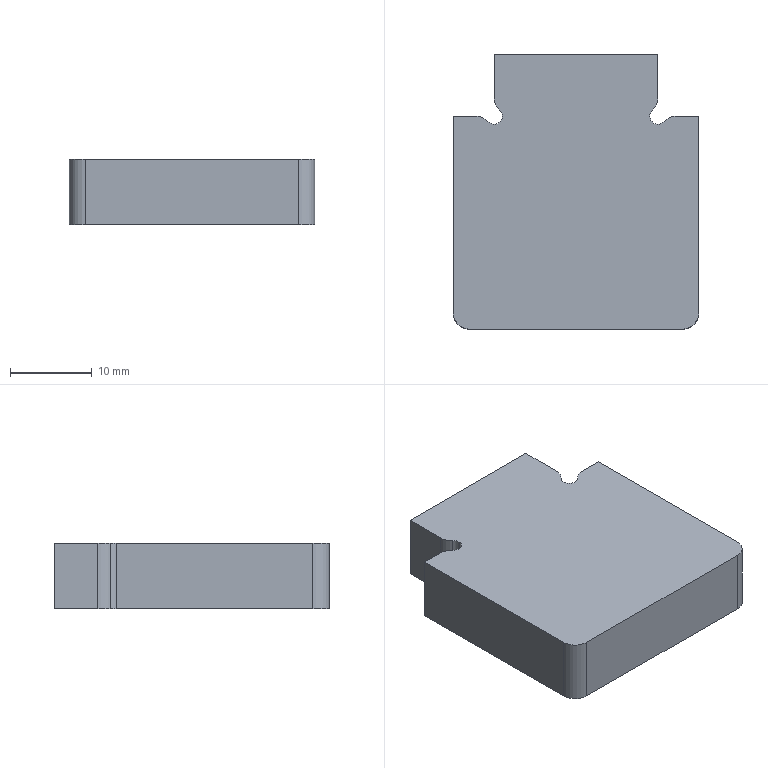Part | SolidWorks | features FlatPattern 1, SMBaseFlange 1, SheetMetal 1 | 1 solid | 19 faces | box 30 x 33.5 x 8 mm | volume 7383 mm3 | plane 10 | cylinder 9 | commonest cylinder face diameters 4 x6 2 x3
STEP:
#1=CARTESIAN_POINT('',(106.89,-100.055,-8.));
#2=VERTEX_POINT('',#1);
#3=CARTESIAN_POINT('',(107.224,-100.8,-8.));
#4=VERTEX_POINT('',#3);
#5=CARTESIAN_POINT('',(106.224,-100.8,-8.));
#6=DIRECTION('',(0.,0.,-1.));
#7=DIRECTION('',(1.,0.,0.));
#8=AXIS2_PLACEMENT_3D('',#5,#6,#7);
#9=CIRCLE('',#8,1.);
#10=EDGE_CURVE('',#2,#4,#9,.T.);
#11=ORIENTED_EDGE('',*,*,#10,.T.);
#12=CARTESIAN_POINT('',(107.224,-100.8,0.));
#13=VERTEX_POINT('',#12);
#14=CARTESIAN_POINT('',(107.224,-100.8,-8.));
#15=DIRECTION('',(0.,0.,1.));
#16=VECTOR('',#15,1000.);
#17=LINE('',#14,#16);
#18=EDGE_CURVE('',#4,#13,#17,.T.);
#19=ORIENTED_EDGE('',*,*,#18,.T.);
#20=CARTESIAN_POINT('',(106.89,-100.055,0.));
#21=VERTEX_POINT('',#20);
#22=CARTESIAN_POINT('',(106.224,-100.8,0.));
#23=DIRECTION('',(0.,0.,-1.));
#24=DIRECTION('',(1.,0.,0.));
#25=AXIS2_PLACEMENT_3D('',#22,#23,#24);
#26=CIRCLE('',#25,1.);
#27=EDGE_CURVE('',#21,#13,#26,.T.);
#28=ORIENTED_EDGE('',*,*,#27,.F.);
#29=CARTESIAN_POINT('',(106.89,-100.055,-8.));
#30=DIRECTION('',(0.,0.,1.));
#31=VECTOR('',#30,1000.);
#32=LINE('',#29,#31);
#33=EDGE_CURVE('',#2,#21,#32,.T.);
#34=ORIENTED_EDGE('',*,*,#33,.F.);
#35=EDGE_LOOP('',(#11,#19,#28,#34));
#36=FACE_OUTER_BOUND('',#35,.T.);
#37=CARTESIAN_POINT('',(106.224,-100.8,-8.));
#38=DIRECTION('',(0.,0.,1.));
#39=DIRECTION('',(1.,0.,0.));
#40=AXIS2_PLACEMENT_3D('',#37,#38,#39);
#41=CYLINDRICAL_SURFACE('',#40,1.);
#42=ADVANCED_FACE('',(#36),#41,.F.);
#43=CARTESIAN_POINT('',(103.988,-100.8,0.));
#44=VERTEX_POINT('',#43);
#45=CARTESIAN_POINT('',(101.224,-100.8,0.));
#46=VERTEX_POINT('',#45);
#47=CARTESIAN_POINT('',(103.988,-100.8,0.));
#48=DIRECTION('',(-1.,0.,0.));
#49=VECTOR('',#48,1000.);
#50=LINE('',#47,#49);
#51=EDGE_CURVE('',#44,#46,#50,.T.);
#52=ORIENTED_EDGE('',*,*,#51,.F.);
#53=CARTESIAN_POINT('',(103.988,-100.8,-8.));
#54=VERTEX_POINT('',#53);
#55=CARTESIAN_POINT('',(103.988,-100.8,-8.));
#56=DIRECTION('',(0.,0.,1.));
#57=VECTOR('',#56,1000.);
#58=LINE('',#55,#57);
#59=EDGE_CURVE('',#54,#44,#58,.T.);
#60=ORIENTED_EDGE('',*,*,#59,.F.);
#61=CARTESIAN_POINT('',(101.224,-100.8,-8.));
#62=VERTEX_POINT('',#61);
#63=CARTESIAN_POINT('',(103.988,-100.8,-8.));
#64=DIRECTION('',(-1.,0.,0.));
#65=VECTOR('',#64,1000.);
#66=LINE('',#63,#65);
#67=EDGE_CURVE('',#54,#62,#66,.T.);
#68=ORIENTED_EDGE('',*,*,#67,.T.);
#69=CARTESIAN_POINT('',(101.224,-100.8,-8.));
#70=DIRECTION('',(0.,0.,1.));
#71=VECTOR('',#70,1000.);
#72=LINE('',#69,#71);
#73=EDGE_CURVE('',#62,#46,#72,.T.);
#74=ORIENTED_EDGE('',*,*,#73,.T.);
#75=EDGE_LOOP('',(#52,#60,#68,#74));
#76=FACE_OUTER_BOUND('',#75,.T.);
#77=CARTESIAN_POINT('',(103.988,-100.8,-8.));
#78=DIRECTION('',(0.,1.,0.));
#79=DIRECTION('',(0.,0.,1.));
#80=AXIS2_PLACEMENT_3D('',#77,#78,#79);
#81=PLANE('',#80);
#82=ADVANCED_FACE('',(#76),#81,.T.);
#83=CARTESIAN_POINT('',(105.478,-101.467,0.));
#84=VERTEX_POINT('',#83);
#85=CARTESIAN_POINT('',(103.988,-102.8,0.));
#86=DIRECTION('',(0.,0.,1.));
#87=DIRECTION('',(1.,0.,0.));
#88=AXIS2_PLACEMENT_3D('',#85,#86,#87);
#89=CIRCLE('',#88,2.);
#90=EDGE_CURVE('',#84,#44,#89,.T.);
#91=ORIENTED_EDGE('',*,*,#90,.F.);
#92=CARTESIAN_POINT('',(105.478,-101.467,-8.));
#93=VERTEX_POINT('',#92);
#94=CARTESIAN_POINT('',(105.478,-101.467,-8.));
#95=DIRECTION('',(0.,0.,1.));
#96=VECTOR('',#95,1000.);
#97=LINE('',#94,#96);
#98=EDGE_CURVE('',#93,#84,#97,.T.);
#99=ORIENTED_EDGE('',*,*,#98,.F.);
#100=CARTESIAN_POINT('',(103.988,-102.8,-8.));
#101=DIRECTION('',(0.,0.,1.));
#102=DIRECTION('',(1.,0.,0.));
#103=AXIS2_PLACEMENT_3D('',#100,#101,#102);
#104=CIRCLE('',#103,2.);
#105=EDGE_CURVE('',#93,#54,#104,.T.);
#106=ORIENTED_EDGE('',*,*,#105,.T.);
#107=ORIENTED_EDGE('',*,*,#59,.T.);
#108=EDGE_LOOP('',(#91,#99,#106,#107));
#109=FACE_OUTER_BOUND('',#108,.T.);
#110=CARTESIAN_POINT('',(103.988,-102.8,-8.));
#111=DIRECTION('',(0.,0.,1.));
#112=DIRECTION('',(1.,0.,0.));
#113=AXIS2_PLACEMENT_3D('',#110,#111,#112);
#114=CYLINDRICAL_SURFACE('',#113,2.);
#115=ADVANCED_FACE('',(#109),#114,.T.);
#116=ORIENTED_EDGE('',*,*,#18,.F.);
#117=CARTESIAN_POINT('',(106.224,-100.8,-8.));
#118=DIRECTION('',(0.,0.,-1.));
#119=DIRECTION('',(1.,0.,0.));
#120=AXIS2_PLACEMENT_3D('',#117,#118,#119);
#121=CIRCLE('',#120,1.);
#122=EDGE_CURVE('',#4,#93,#121,.T.);
#123=ORIENTED_EDGE('',*,*,#122,.T.);
#124=ORIENTED_EDGE('',*,*,#98,.T.);
#125=CARTESIAN_POINT('',(106.224,-100.8,0.));
#126=DIRECTION('',(0.,0.,-1.));
#127=DIRECTION('',(1.,0.,0.));
#128=AXIS2_PLACEMENT_3D('',#125,#126,#127);
#129=CIRCLE('',#128,1.);
#130=EDGE_CURVE('',#13,#84,#129,.T.);
#131=ORIENTED_EDGE('',*,*,#130,.F.);
#132=EDGE_LOOP('',(#116,#123,#124,#131));
#133=FACE_OUTER_BOUND('',#132,.T.);
#134=CARTESIAN_POINT('',(106.224,-100.8,-8.));
#135=DIRECTION('',(0.,0.,1.));
#136=DIRECTION('',(1.,0.,0.));
#137=AXIS2_PLACEMENT_3D('',#134,#135,#136);
#138=CYLINDRICAL_SURFACE('',#137,1.);
#139=ADVANCED_FACE('',(#133),#138,.F.);
#140=CARTESIAN_POINT('',(106.224,-98.564,0.));
#141=VERTEX_POINT('',#140);
#142=CARTESIAN_POINT('',(108.224,-98.564,0.));
#143=DIRECTION('',(0.,0.,1.));
#144=DIRECTION('',(-1.,0.,0.));
#145=AXIS2_PLACEMENT_3D('',#142,#143,#144);
#146=CIRCLE('',#145,2.);
#147=EDGE_CURVE('',#141,#21,#146,.T.);
#148=ORIENTED_EDGE('',*,*,#147,.F.);
#149=CARTESIAN_POINT('',(106.224,-98.564,-8.));
#150=VERTEX_POINT('',#149);
#151=CARTESIAN_POINT('',(106.224,-98.564,-8.));
#152=DIRECTION('',(0.,0.,1.));
#153=VECTOR('',#152,1000.);
#154=LINE('',#151,#153);
#155=EDGE_CURVE('',#150,#141,#154,.T.);
#156=ORIENTED_EDGE('',*,*,#155,.F.);
#157=CARTESIAN_POINT('',(108.224,-98.564,-8.));
#158=DIRECTION('',(0.,0.,1.));
#159=DIRECTION('',(-1.,0.,0.));
#160=AXIS2_PLACEMENT_3D('',#157,#158,#159);
#161=CIRCLE('',#160,2.);
#162=EDGE_CURVE('',#150,#2,#161,.T.);
#163=ORIENTED_EDGE('',*,*,#162,.T.);
#164=ORIENTED_EDGE('',*,*,#33,.T.);
#165=EDGE_LOOP('',(#148,#156,#163,#164));
#166=FACE_OUTER_BOUND('',#165,.T.);
#167=CARTESIAN_POINT('',(108.224,-98.564,-8.));
#168=DIRECTION('',(0.,0.,1.));
#169=DIRECTION('',(1.,0.,0.));
#170=AXIS2_PLACEMENT_3D('',#167,#168,#169);
#171=CYLINDRICAL_SURFACE('',#170,2.);
#172=ADVANCED_FACE('',(#166),#171,.T.);
#173=CARTESIAN_POINT('',(106.224,-93.3,0.));
#174=VERTEX_POINT('',#173);
#175=CARTESIAN_POINT('',(106.224,-93.3,0.));
#176=DIRECTION('',(0.,-1.,0.));
#177=VECTOR('',#176,1000.);
#178=LINE('',#175,#177);
#179=EDGE_CURVE('',#174,#141,#178,.T.);
#180=ORIENTED_EDGE('',*,*,#179,.F.);
#181=CARTESIAN_POINT('',(106.224,-93.3,-8.));
#182=VERTEX_POINT('',#181);
#183=CARTESIAN_POINT('',(106.224,-93.3,-8.));
#184=DIRECTION('',(0.,0.,1.));
#185=VECTOR('',#184,1000.);
#186=LINE('',#183,#185);
#187=EDGE_CURVE('',#182,#174,#186,.T.);
#188=ORIENTED_EDGE('',*,*,#187,.F.);
#189=CARTESIAN_POINT('',(106.224,-93.3,-8.));
#190=DIRECTION('',(0.,-1.,0.));
#191=VECTOR('',#190,1000.);
#192=LINE('',#189,#191);
#193=EDGE_CURVE('',#182,#150,#192,.T.);
#194=ORIENTED_EDGE('',*,*,#193,.T.);
#195=ORIENTED_EDGE('',*,*,#155,.T.);
#196=EDGE_LOOP('',(#180,#188,#194,#195));
#197=FACE_OUTER_BOUND('',#196,.T.);
#198=CARTESIAN_POINT('',(106.224,-93.3,-8.));
#199=DIRECTION('',(-1.,0.,0.));
#200=DIRECTION('',(0.,0.,1.));
#201=AXIS2_PLACEMENT_3D('',#198,#199,#200);
#202=PLANE('',#201);
#203=ADVANCED_FACE('',(#197),#202,.T.);
#204=CARTESIAN_POINT('',(126.224,-93.3,0.));
#205=VERTEX_POINT('',#204);
#206=CARTESIAN_POINT('',(126.224,-93.3,0.));
#207=DIRECTION('',(-1.,0.,0.));
#208=VECTOR('',#207,1000.);
#209=LINE('',#206,#208);
#210=EDGE_CURVE('',#205,#174,#209,.T.);
#211=ORIENTED_EDGE('',*,*,#210,.F.);
#212=CARTESIAN_POINT('',(126.224,-93.3,-8.));
#213=VERTEX_POINT('',#212);
#214=CARTESIAN_POINT('',(126.224,-93.3,-8.));
#215=DIRECTION('',(0.,0.,1.));
#216=VECTOR('',#215,1000.);
#217=LINE('',#214,#216);
#218=EDGE_CURVE('',#213,#205,#217,.T.);
#219=ORIENTED_EDGE('',*,*,#218,.F.);
#220=CARTESIAN_POINT('',(126.224,-93.3,-8.));
#221=DIRECTION('',(-1.,0.,0.));
#222=VECTOR('',#221,1000.);
#223=LINE('',#220,#222);
#224=EDGE_CURVE('',#213,#182,#223,.T.);
#225=ORIENTED_EDGE('',*,*,#224,.T.);
#226=ORIENTED_EDGE('',*,*,#187,.T.);
#227=EDGE_LOOP('',(#211,#219,#225,#226));
#228=FACE_OUTER_BOUND('',#227,.T.);
#229=CARTESIAN_POINT('',(126.224,-93.3,-8.));
#230=DIRECTION('',(0.,1.,0.));
#231=DIRECTION('',(0.,0.,1.));
#232=AXIS2_PLACEMENT_3D('',#229,#230,#231);
#233=PLANE('',#232);
#234=ADVANCED_FACE('',(#228),#233,.T.);
#235=CARTESIAN_POINT('',(126.224,-98.564,0.));
#236=VERTEX_POINT('',#235);
#237=CARTESIAN_POINT('',(126.224,-98.564,0.));
#238=DIRECTION('',(0.,1.,0.));
#239=VECTOR('',#238,1000.);
#240=LINE('',#237,#239);
#241=EDGE_CURVE('',#236,#205,#240,.T.);
#242=ORIENTED_EDGE('',*,*,#241,.F.);
#243=CARTESIAN_POINT('',(126.224,-98.564,-8.));
#244=VERTEX_POINT('',#243);
#245=CARTESIAN_POINT('',(126.224,-98.564,-8.));
#246=DIRECTION('',(0.,0.,1.));
#247=VECTOR('',#246,1000.);
#248=LINE('',#245,#247);
#249=EDGE_CURVE('',#244,#236,#248,.T.);
#250=ORIENTED_EDGE('',*,*,#249,.F.);
#251=CARTESIAN_POINT('',(126.224,-98.564,-8.));
#252=DIRECTION('',(0.,1.,0.));
#253=VECTOR('',#252,1000.);
#254=LINE('',#251,#253);
#255=EDGE_CURVE('',#244,#213,#254,.T.);
#256=ORIENTED_EDGE('',*,*,#255,.T.);
#257=ORIENTED_EDGE('',*,*,#218,.T.);
#258=EDGE_LOOP('',(#242,#250,#256,#257));
#259=FACE_OUTER_BOUND('',#258,.T.);
#260=CARTESIAN_POINT('',(126.224,-98.564,-8.));
#261=DIRECTION('',(1.,0.,0.));
#262=DIRECTION('',(0.,0.,-1.));
#263=AXIS2_PLACEMENT_3D('',#260,#261,#262);
#264=PLANE('',#263);
#265=ADVANCED_FACE('',(#259),#264,.T.);
#266=CARTESIAN_POINT('',(125.557,-100.055,0.));
#267=VERTEX_POINT('',#266);
#268=CARTESIAN_POINT('',(124.224,-98.564,0.));
#269=DIRECTION('',(0.,0.,1.));
#270=DIRECTION('',(1.,0.,0.));
#271=AXIS2_PLACEMENT_3D('',#268,#269,#270);
#272=CIRCLE('',#271,2.);
#273=EDGE_CURVE('',#267,#236,#272,.T.);
#274=ORIENTED_EDGE('',*,*,#273,.F.);
#275=CARTESIAN_POINT('',(125.557,-100.055,-8.));
#276=VERTEX_POINT('',#275);
#277=CARTESIAN_POINT('',(125.557,-100.055,-8.));
#278=DIRECTION('',(0.,0.,1.));
#279=VECTOR('',#278,1000.);
#280=LINE('',#277,#279);
#281=EDGE_CURVE('',#276,#267,#280,.T.);
#282=ORIENTED_EDGE('',*,*,#281,.F.);
#283=CARTESIAN_POINT('',(124.224,-98.564,-8.));
#284=DIRECTION('',(0.,0.,1.));
#285=DIRECTION('',(1.,0.,0.));
#286=AXIS2_PLACEMENT_3D('',#283,#284,#285);
#287=CIRCLE('',#286,2.);
#288=EDGE_CURVE('',#276,#244,#287,.T.);
#289=ORIENTED_EDGE('',*,*,#288,.T.);
#290=ORIENTED_EDGE('',*,*,#249,.T.);
#291=EDGE_LOOP('',(#274,#282,#289,#290));
#292=FACE_OUTER_BOUND('',#291,.T.);
#293=CARTESIAN_POINT('',(124.224,-98.564,-8.));
#294=DIRECTION('',(0.,0.,1.));
#295=DIRECTION('',(1.,0.,0.));
#296=AXIS2_PLACEMENT_3D('',#293,#294,#295);
#297=CYLINDRICAL_SURFACE('',#296,2.);
#298=ADVANCED_FACE('',(#292),#297,.T.);
#299=CARTESIAN_POINT('',(126.969,-101.467,0.));
#300=VERTEX_POINT('',#299);
#301=CARTESIAN_POINT('',(126.224,-100.8,0.));
#302=DIRECTION('',(0.,0.,-1.));
#303=DIRECTION('',(1.,0.,0.));
#304=AXIS2_PLACEMENT_3D('',#301,#302,#303);
#305=CIRCLE('',#304,1.);
#306=EDGE_CURVE('',#300,#267,#305,.T.);
#307=ORIENTED_EDGE('',*,*,#306,.F.);
#308=CARTESIAN_POINT('',(126.969,-101.467,-8.));
#309=VERTEX_POINT('',#308);
#310=CARTESIAN_POINT('',(126.969,-101.467,-8.));
#311=DIRECTION('',(0.,0.,1.));
#312=VECTOR('',#311,1000.);
#313=LINE('',#310,#312);
#314=EDGE_CURVE('',#309,#300,#313,.T.);
#315=ORIENTED_EDGE('',*,*,#314,.F.);
#316=CARTESIAN_POINT('',(126.224,-100.8,-8.));
#317=DIRECTION('',(0.,0.,-1.));
#318=DIRECTION('',(1.,0.,0.));
#319=AXIS2_PLACEMENT_3D('',#316,#317,#318);
#320=CIRCLE('',#319,1.);
#321=EDGE_CURVE('',#309,#276,#320,.T.);
#322=ORIENTED_EDGE('',*,*,#321,.T.);
#323=ORIENTED_EDGE('',*,*,#281,.T.);
#324=EDGE_LOOP('',(#307,#315,#322,#323));
#325=FACE_OUTER_BOUND('',#324,.T.);
#326=CARTESIAN_POINT('',(126.224,-100.8,-8.));
#327=DIRECTION('',(0.,0.,1.));
#328=DIRECTION('',(1.,0.,0.));
#329=AXIS2_PLACEMENT_3D('',#326,#327,#328);
#330=CYLINDRICAL_SURFACE('',#329,1.);
#331=ADVANCED_FACE('',(#325),#330,.F.);
#332=CARTESIAN_POINT('',(128.46,-100.8,0.));
#333=VERTEX_POINT('',#332);
#334=CARTESIAN_POINT('',(128.46,-102.8,0.));
#335=DIRECTION('',(0.,0.,1.));
#336=DIRECTION('',(-1.,0.,0.));
#337=AXIS2_PLACEMENT_3D('',#334,#335,#336);
#338=CIRCLE('',#337,2.);
#339=EDGE_CURVE('',#333,#300,#338,.T.);
#340=ORIENTED_EDGE('',*,*,#339,.F.);
#341=CARTESIAN_POINT('',(128.46,-100.8,-8.));
#342=VERTEX_POINT('',#341);
#343=CARTESIAN_POINT('',(128.46,-100.8,-8.));
#344=DIRECTION('',(0.,0.,1.));
#345=VECTOR('',#344,1000.);
#346=LINE('',#343,#345);
#347=EDGE_CURVE('',#342,#333,#346,.T.);
#348=ORIENTED_EDGE('',*,*,#347,.F.);
#349=CARTESIAN_POINT('',(128.46,-102.8,-8.));
#350=DIRECTION('',(0.,0.,1.));
#351=DIRECTION('',(-1.,0.,0.));
#352=AXIS2_PLACEMENT_3D('',#349,#350,#351);
#353=CIRCLE('',#352,2.);
#354=EDGE_CURVE('',#342,#309,#353,.T.);
#355=ORIENTED_EDGE('',*,*,#354,.T.);
#356=ORIENTED_EDGE('',*,*,#314,.T.);
#357=EDGE_LOOP('',(#340,#348,#355,#356));
#358=FACE_OUTER_BOUND('',#357,.T.);
#359=CARTESIAN_POINT('',(128.46,-102.8,-8.));
#360=DIRECTION('',(0.,0.,1.));
#361=DIRECTION('',(1.,0.,0.));
#362=AXIS2_PLACEMENT_3D('',#359,#360,#361);
#363=CYLINDRICAL_SURFACE('',#362,2.);
#364=ADVANCED_FACE('',(#358),#363,.T.);
#365=CARTESIAN_POINT('',(131.224,-100.8,0.));
#366=VERTEX_POINT('',#365);
#367=CARTESIAN_POINT('',(131.224,-100.8,0.));
#368=DIRECTION('',(-1.,0.,0.));
#369=VECTOR('',#368,1000.);
#370=LINE('',#367,#369);
#371=EDGE_CURVE('',#366,#333,#370,.T.);
#372=ORIENTED_EDGE('',*,*,#371,.F.);
#373=CARTESIAN_POINT('',(131.224,-100.8,-8.));
#374=VERTEX_POINT('',#373);
#375=CARTESIAN_POINT('',(131.224,-100.8,-8.));
#376=DIRECTION('',(0.,0.,1.));
#377=VECTOR('',#376,1000.);
#378=LINE('',#375,#377);
#379=EDGE_CURVE('',#374,#366,#378,.T.);
#380=ORIENTED_EDGE('',*,*,#379,.F.);
#381=CARTESIAN_POINT('',(131.224,-100.8,-8.));
#382=DIRECTION('',(-1.,0.,0.));
#383=VECTOR('',#382,1000.);
#384=LINE('',#381,#383);
#385=EDGE_CURVE('',#374,#342,#384,.T.);
#386=ORIENTED_EDGE('',*,*,#385,.T.);
#387=ORIENTED_EDGE('',*,*,#347,.T.);
#388=EDGE_LOOP('',(#372,#380,#386,#387));
#389=FACE_OUTER_BOUND('',#388,.T.);
#390=CARTESIAN_POINT('',(131.224,-100.8,-8.));
#391=DIRECTION('',(0.,1.,0.));
#392=DIRECTION('',(0.,0.,1.));
#393=AXIS2_PLACEMENT_3D('',#390,#391,#392);
#394=PLANE('',#393);
#395=ADVANCED_FACE('',(#389),#394,.T.);
#396=CARTESIAN_POINT('',(131.224,-124.8,0.));
#397=VERTEX_POINT('',#396);
#398=CARTESIAN_POINT('',(131.224,-124.8,0.));
#399=DIRECTION('',(0.,1.,0.));
#400=VECTOR('',#399,1000.);
#401=LINE('',#398,#400);
#402=EDGE_CURVE('',#397,#366,#401,.T.);
#403=ORIENTED_EDGE('',*,*,#402,.F.);
#404=CARTESIAN_POINT('',(131.224,-124.8,-8.));
#405=VERTEX_POINT('',#404);
#406=CARTESIAN_POINT('',(131.224,-124.8,-8.));
#407=DIRECTION('',(0.,0.,1.));
#408=VECTOR('',#407,1000.);
#409=LINE('',#406,#408);
#410=EDGE_CURVE('',#405,#397,#409,.T.);
#411=ORIENTED_EDGE('',*,*,#410,.F.);
#412=CARTESIAN_POINT('',(131.224,-124.8,-8.));
#413=DIRECTION('',(0.,1.,0.));
#414=VECTOR('',#413,1000.);
#415=LINE('',#412,#414);
#416=EDGE_CURVE('',#405,#374,#415,.T.);
#417=ORIENTED_EDGE('',*,*,#416,.T.);
#418=ORIENTED_EDGE('',*,*,#379,.T.);
#419=EDGE_LOOP('',(#403,#411,#417,#418));
#420=FACE_OUTER_BOUND('',#419,.T.);
#421=CARTESIAN_POINT('',(131.224,-124.8,-8.));
#422=DIRECTION('',(1.,0.,0.));
#423=DIRECTION('',(0.,0.,-1.));
#424=AXIS2_PLACEMENT_3D('',#421,#422,#423);
#425=PLANE('',#424);
#426=ADVANCED_FACE('',(#420),#425,.T.);
#427=CARTESIAN_POINT('',(129.224,-126.8,0.));
#428=VERTEX_POINT('',#427);
#429=CARTESIAN_POINT('',(129.224,-124.8,0.));
#430=DIRECTION('',(0.,0.,1.));
#431=DIRECTION('',(1.,0.,0.));
#432=AXIS2_PLACEMENT_3D('',#429,#430,#431);
#433=CIRCLE('',#432,2.);
#434=EDGE_CURVE('',#428,#397,#433,.T.);
#435=ORIENTED_EDGE('',*,*,#434,.F.);
#436=CARTESIAN_POINT('',(129.224,-126.8,-8.));
#437=VERTEX_POINT('',#436);
#438=CARTESIAN_POINT('',(129.224,-126.8,-8.));
#439=DIRECTION('',(0.,0.,1.));
#440=VECTOR('',#439,1000.);
#441=LINE('',#438,#440);
#442=EDGE_CURVE('',#437,#428,#441,.T.);
#443=ORIENTED_EDGE('',*,*,#442,.F.);
#444=CARTESIAN_POINT('',(129.224,-124.8,-8.));
#445=DIRECTION('',(0.,0.,1.));
#446=DIRECTION('',(1.,0.,0.));
#447=AXIS2_PLACEMENT_3D('',#444,#445,#446);
#448=CIRCLE('',#447,2.);
#449=EDGE_CURVE('',#437,#405,#448,.T.);
#450=ORIENTED_EDGE('',*,*,#449,.T.);
#451=ORIENTED_EDGE('',*,*,#410,.T.);
#452=EDGE_LOOP('',(#435,#443,#450,#451));
#453=FACE_OUTER_BOUND('',#452,.T.);
#454=CARTESIAN_POINT('',(129.224,-124.8,-8.));
#455=DIRECTION('',(0.,0.,1.));
#456=DIRECTION('',(1.,0.,0.));
#457=AXIS2_PLACEMENT_3D('',#454,#455,#456);
#458=CYLINDRICAL_SURFACE('',#457,2.);
#459=ADVANCED_FACE('',(#453),#458,.T.);
#460=CARTESIAN_POINT('',(103.224,-126.8,0.));
#461=VERTEX_POINT('',#460);
#462=CARTESIAN_POINT('',(103.224,-126.8,0.));
#463=DIRECTION('',(1.,0.,0.));
#464=VECTOR('',#463,1000.);
#465=LINE('',#462,#464);
#466=EDGE_CURVE('',#461,#428,#465,.T.);
#467=ORIENTED_EDGE('',*,*,#466,.F.);
#468=CARTESIAN_POINT('',(103.224,-126.8,-8.));
#469=VERTEX_POINT('',#468);
#470=CARTESIAN_POINT('',(103.224,-126.8,-8.));
#471=DIRECTION('',(0.,0.,1.));
#472=VECTOR('',#471,1000.);
#473=LINE('',#470,#472);
#474=EDGE_CURVE('',#469,#461,#473,.T.);
#475=ORIENTED_EDGE('',*,*,#474,.F.);
#476=CARTESIAN_POINT('',(103.224,-126.8,-8.));
#477=DIRECTION('',(1.,0.,0.));
#478=VECTOR('',#477,1000.);
#479=LINE('',#476,#478);
#480=EDGE_CURVE('',#469,#437,#479,.T.);
#481=ORIENTED_EDGE('',*,*,#480,.T.);
#482=ORIENTED_EDGE('',*,*,#442,.T.);
#483=EDGE_LOOP('',(#467,#475,#481,#482));
#484=FACE_OUTER_BOUND('',#483,.T.);
#485=CARTESIAN_POINT('',(103.224,-126.8,-8.));
#486=DIRECTION('',(0.,-1.,0.));
#487=DIRECTION('',(0.,0.,-1.));
#488=AXIS2_PLACEMENT_3D('',#485,#486,#487);
#489=PLANE('',#488);
#490=ADVANCED_FACE('',(#484),#489,.T.);
#491=CARTESIAN_POINT('',(101.224,-124.8,0.));
#492=VERTEX_POINT('',#491);
#493=CARTESIAN_POINT('',(103.224,-124.8,0.));
#494=DIRECTION('',(0.,0.,1.));
#495=DIRECTION('',(1.,0.,0.));
#496=AXIS2_PLACEMENT_3D('',#493,#494,#495);
#497=CIRCLE('',#496,2.);
#498=EDGE_CURVE('',#492,#461,#497,.T.);
#499=ORIENTED_EDGE('',*,*,#498,.F.);
#500=CARTESIAN_POINT('',(101.224,-124.8,-8.));
#501=VERTEX_POINT('',#500);
#502=CARTESIAN_POINT('',(101.224,-124.8,-8.));
#503=DIRECTION('',(0.,0.,1.));
#504=VECTOR('',#503,1000.);
#505=LINE('',#502,#504);
#506=EDGE_CURVE('',#501,#492,#505,.T.);
#507=ORIENTED_EDGE('',*,*,#506,.F.);
#508=CARTESIAN_POINT('',(103.224,-124.8,-8.));
#509=DIRECTION('',(0.,0.,1.));
#510=DIRECTION('',(1.,0.,0.));
#511=AXIS2_PLACEMENT_3D('',#508,#509,#510);
#512=CIRCLE('',#511,2.);
#513=EDGE_CURVE('',#501,#469,#512,.T.);
#514=ORIENTED_EDGE('',*,*,#513,.T.);
#515=ORIENTED_EDGE('',*,*,#474,.T.);
#516=EDGE_LOOP('',(#499,#507,#514,#515));
#517=FACE_OUTER_BOUND('',#516,.T.);
#518=CARTESIAN_POINT('',(103.224,-124.8,-8.));
#519=DIRECTION('',(0.,0.,1.));
#520=DIRECTION('',(1.,0.,0.));
#521=AXIS2_PLACEMENT_3D('',#518,#519,#520);
#522=CYLINDRICAL_SURFACE('',#521,2.);
#523=ADVANCED_FACE('',(#517),#522,.T.);
#524=CARTESIAN_POINT('',(101.224,-100.8,0.));
#525=DIRECTION('',(0.,-1.,0.));
#526=VECTOR('',#525,1000.);
#527=LINE('',#524,#526);
#528=EDGE_CURVE('',#46,#492,#527,.T.);
#529=ORIENTED_EDGE('',*,*,#528,.F.);
#530=ORIENTED_EDGE('',*,*,#73,.F.);
#531=CARTESIAN_POINT('',(101.224,-100.8,-8.));
#532=DIRECTION('',(0.,-1.,0.));
#533=VECTOR('',#532,1000.);
#534=LINE('',#531,#533);
#535=EDGE_CURVE('',#62,#501,#534,.T.);
#536=ORIENTED_EDGE('',*,*,#535,.T.);
#537=ORIENTED_EDGE('',*,*,#506,.T.);
#538=EDGE_LOOP('',(#529,#530,#536,#537));
#539=FACE_OUTER_BOUND('',#538,.T.);
#540=CARTESIAN_POINT('',(101.224,-100.8,-8.));
#541=DIRECTION('',(-1.,0.,0.));
#542=DIRECTION('',(0.,-1.,0.));
#543=AXIS2_PLACEMENT_3D('',#540,#541,#542);
#544=PLANE('',#543);
#545=ADVANCED_FACE('',(#539),#544,.T.);
#546=ORIENTED_EDGE('',*,*,#67,.F.);
#547=ORIENTED_EDGE('',*,*,#105,.F.);
#548=ORIENTED_EDGE('',*,*,#122,.F.);
#549=ORIENTED_EDGE('',*,*,#10,.F.);
#550=ORIENTED_EDGE('',*,*,#162,.F.);
#551=ORIENTED_EDGE('',*,*,#193,.F.);
#552=ORIENTED_EDGE('',*,*,#224,.F.);
#553=ORIENTED_EDGE('',*,*,#255,.F.);
#554=ORIENTED_EDGE('',*,*,#288,.F.);
#555=ORIENTED_EDGE('',*,*,#321,.F.);
#556=ORIENTED_EDGE('',*,*,#354,.F.);
#557=ORIENTED_EDGE('',*,*,#385,.F.);
#558=ORIENTED_EDGE('',*,*,#416,.F.);
#559=ORIENTED_EDGE('',*,*,#449,.F.);
#560=ORIENTED_EDGE('',*,*,#480,.F.);
#561=ORIENTED_EDGE('',*,*,#513,.F.);
#562=ORIENTED_EDGE('',*,*,#535,.F.);
#563=EDGE_LOOP('',(#546,#547,#548,#549,#550,#551,#552,#553,#554,#555,#556,#557,#558,#559,#560,#561,#562));
#564=FACE_OUTER_BOUND('',#563,.T.);
#565=CARTESIAN_POINT('',(103.224,-124.8,-8.));
#566=DIRECTION('',(0.,0.,1.));
#567=DIRECTION('',(1.,0.,0.));
#568=AXIS2_PLACEMENT_3D('',#565,#566,#567);
#569=PLANE('',#568);
#570=ADVANCED_FACE('',(#564),#569,.F.);
#571=ORIENTED_EDGE('',*,*,#51,.T.);
#572=ORIENTED_EDGE('',*,*,#528,.T.);
#573=ORIENTED_EDGE('',*,*,#498,.T.);
#574=ORIENTED_EDGE('',*,*,#466,.T.);
#575=ORIENTED_EDGE('',*,*,#434,.T.);
#576=ORIENTED_EDGE('',*,*,#402,.T.);
#577=ORIENTED_EDGE('',*,*,#371,.T.);
#578=ORIENTED_EDGE('',*,*,#339,.T.);
#579=ORIENTED_EDGE('',*,*,#306,.T.);
#580=ORIENTED_EDGE('',*,*,#273,.T.);
#581=ORIENTED_EDGE('',*,*,#241,.T.);
#582=ORIENTED_EDGE('',*,*,#210,.T.);
#583=ORIENTED_EDGE('',*,*,#179,.T.);
#584=ORIENTED_EDGE('',*,*,#147,.T.);
#585=ORIENTED_EDGE('',*,*,#27,.T.);
#586=ORIENTED_EDGE('',*,*,#130,.T.);
#587=ORIENTED_EDGE('',*,*,#90,.T.);
#588=EDGE_LOOP('',(#571,#572,#573,#574,#575,#576,#577,#578,#579,#580,#581,#582,#583,#584,#585,#586,#587));
#589=FACE_OUTER_BOUND('',#588,.T.);
#590=CARTESIAN_POINT('',(103.224,-124.8,0.));
#591=DIRECTION('',(0.,0.,1.));
#592=DIRECTION('',(1.,0.,0.));
#593=AXIS2_PLACEMENT_3D('',#590,#591,#592);
#594=PLANE('',#593);
#595=ADVANCED_FACE('',(#589),#594,.T.);
#596=CLOSED_SHELL('',(#42,#82,#115,#139,#172,#203,#234,#265,#298,#331,#364,#395,#426,#459,#490,#523,#545,#570,#595));
#597=MANIFOLD_SOLID_BREP('',#596);
#598=CARTESIAN_POINT('',(0.,0.,0.));
#599=DIRECTION('',(0.,0.,1.));
#600=DIRECTION('',(1.,0.,0.));
#601=AXIS2_PLACEMENT_3D('',#598,#599,#600);
#602=(LENGTH_UNIT()NAMED_UNIT(*)SI_UNIT(.MILLI.,.METRE.));
#603=UNCERTAINTY_MEASURE_WITH_UNIT(LENGTH_MEASURE(0.00001),#602,'','');
#604=(NAMED_UNIT(*)PLANE_ANGLE_UNIT()SI_UNIT($,.RADIAN.));
#605=(NAMED_UNIT(*)SI_UNIT($,.STERADIAN.)SOLID_ANGLE_UNIT());
#606=(GEOMETRIC_REPRESENTATION_CONTEXT(3)GLOBAL_UNCERTAINTY_ASSIGNED_CONTEXT((#603))GLOBAL_UNIT_ASSIGNED_CONTEXT((#602,#604,#605))REPRESENTATION_CONTEXT('',''));
#607=ADVANCED_BREP_SHAPE_REPRESENTATION('',(#597,#601),#606);